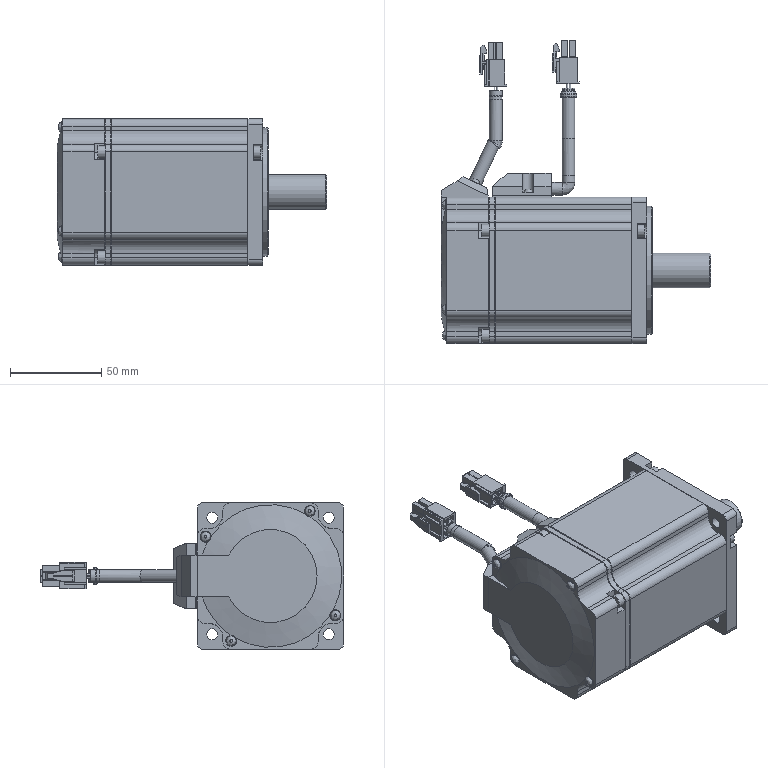Part | NX | 7 solids | 683 faces | box 147.2 x 165.8 x 80 mm | volume 673452 mm3 | plane 487 | cylinder 169 | spline 14 | cone 13 | commonest cylinder face diameters 8 x44 15 x24 0.6 x18 7 x15 6 x14 1 x10